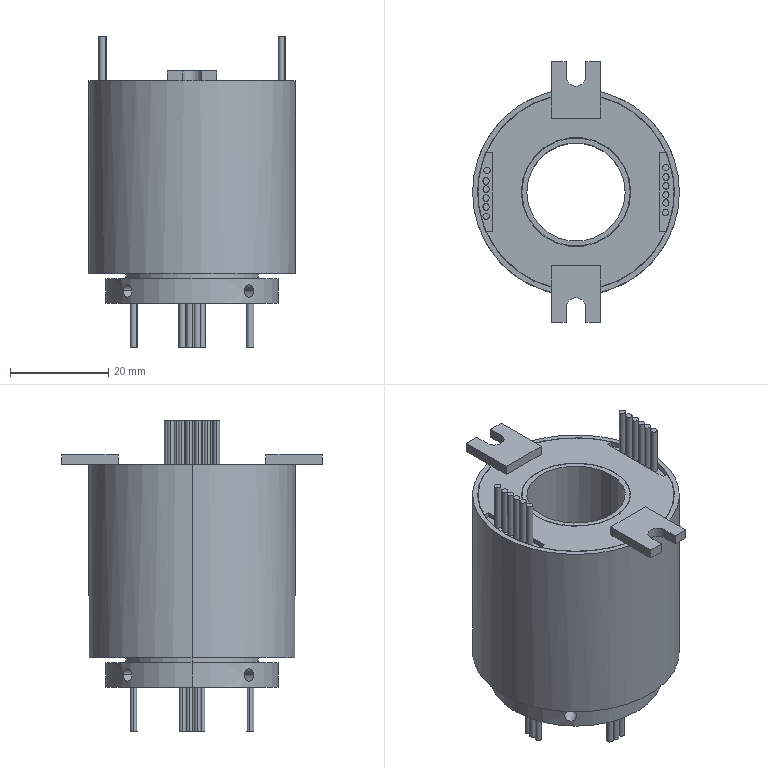Part | SolidWorks | features BaseBody 1 | 1 solid | 171 faces | box 42 x 53 x 63.2 mm | volume 45858 mm3 | cylinder 104 | plane 67 | commonest cylinder face diameters 1.3 x48 1.5 x12 22.5 x9 2.5 x8 25.5 x5 40 x4